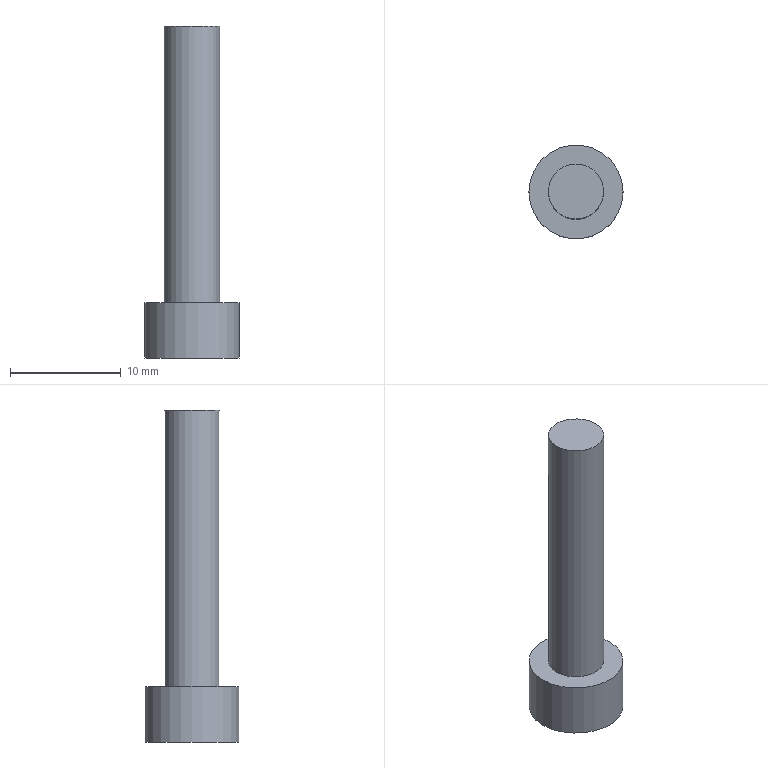Part | STEP file | 1 solid | 12 faces | box 8.5 x 8.5 x 30 mm | volume 728.873 mm3 | plane 10 | cylinder 2 | commonest cylinder face diameters 5 x1 8.5 x1
STEP:
#1=CARTESIAN_POINT('',(0.,0.,0.));
#2=DIRECTION('',(0.,0.,1.));
#3=DIRECTION('',(1.,0.,0.));
#4=AXIS2_PLACEMENT_3D('',#1,#2,#3);
#5=CARTESIAN_POINT('',(1182.997,385.855,-56.381));
#6=VERTEX_POINT('',#5);
#7=CARTESIAN_POINT('',(1187.247,385.855,-56.381));
#8=DIRECTION('',(0.,0.,-1.));
#9=DIRECTION('',(-1.,0.,0.));
#10=AXIS2_PLACEMENT_3D('',#7,#8,#9);
#11=CIRCLE('',#10,4.25);
#12=CARTESIAN_POINT('',(1182.997,385.855,-56.381));
#13=DIRECTION('',(0.,0.,1.));
#14=DIRECTION('',(1.,0.,0.));
#15=AXIS2_PLACEMENT_3D('',#12,#13,#14);
#16=PLANE('',#15);
#17=CARTESIAN_POINT('',(0.,0.));
#18=CARTESIAN_POINT('',(0.,7.361));
#19=CARTESIAN_POINT('',(6.375,3.681));
#20=CARTESIAN_POINT('',(12.75,0.));
#21=CARTESIAN_POINT('',(6.375,-3.681));
#22=CARTESIAN_POINT('',(0.,-7.361));
#23=CARTESIAN_POINT('',(0.,0.));
#24=(BOUNDED_CURVE()B_SPLINE_CURVE(2,(#17,#18,#19,#20,#21,#22,#23),.UNSPECIFIED.,.T.,.F.)B_SPLINE_CURVE_WITH_KNOTS((1,2,2,2,2,1),(-2.094,0.,2.094,4.189,6.283,8.378),.UNSPECIFIED.)CURVE()GEOMETRIC_REPRESENTATION_ITEM()RATIONAL_B_SPLINE_CURVE((1.,0.5,1.,0.5,1.,0.5,1.))REPRESENTATION_ITEM(''));
#25=(GEOMETRIC_REPRESENTATION_CONTEXT(2)PARAMETRIC_REPRESENTATION_CONTEXT()REPRESENTATION_CONTEXT('',''));
#26=DEFINITIONAL_REPRESENTATION('',(#24),#25);
#27=PCURVE('',#16,#26);
#28=CARTESIAN_POINT('',(1187.247,385.855,-19.981));
#29=DIRECTION('',(0.,0.,-1.));
#30=DIRECTION('',(-1.,0.,0.));
#31=AXIS2_PLACEMENT_3D('',#28,#29,#30);
#32=CYLINDRICAL_SURFACE('',#31,4.25);
#33=CARTESIAN_POINT('',(0.,36.4));
#34=DIRECTION('',(1.,0.));
#35=VECTOR('',#34,1.);
#36=LINE('',#33,#35);
#37=(GEOMETRIC_REPRESENTATION_CONTEXT(2)PARAMETRIC_REPRESENTATION_CONTEXT()REPRESENTATION_CONTEXT('',''));
#38=DEFINITIONAL_REPRESENTATION('',(#36),#37);
#39=PCURVE('',#32,#38);
#40=SURFACE_CURVE('',#11,(#27,#39),.PCURVE_S1.);
#41=EDGE_CURVE('',#6,#6,#40,.T.);
#42=ORIENTED_EDGE('',*,*,#41,.T.);
#43=EDGE_LOOP('',(#42));
#44=FACE_BOUND('',#43,.T.);
#45=CARTESIAN_POINT('',(1188.402,387.855,-56.381));
#46=VERTEX_POINT('',#45);
#47=CARTESIAN_POINT('',(1186.092,387.855,-56.381));
#48=VERTEX_POINT('',#47);
#49=CARTESIAN_POINT('',(1188.402,387.855,-56.381));
#50=DIRECTION('',(-1.,0.,0.));
#51=VECTOR('',#50,1.);
#52=LINE('',#49,#51);
#53=CARTESIAN_POINT('',(5.405,2.));
#54=DIRECTION('',(-1.,0.));
#55=VECTOR('',#54,1.);
#56=LINE('',#53,#55);
#57=(GEOMETRIC_REPRESENTATION_CONTEXT(2)PARAMETRIC_REPRESENTATION_CONTEXT()REPRESENTATION_CONTEXT('',''));
#58=DEFINITIONAL_REPRESENTATION('',(#56),#57);
#59=PCURVE('',#16,#58);
#60=CARTESIAN_POINT('',(1188.402,387.855,-53.081));
#61=DIRECTION('',(0.,-1.,0.));
#62=DIRECTION('',(-1.,0.,0.));
#63=AXIS2_PLACEMENT_3D('',#60,#61,#62);
#64=PLANE('',#63);
#65=CARTESIAN_POINT('',(0.,3.3));
#66=DIRECTION('',(1.,0.));
#67=VECTOR('',#66,1.);
#68=LINE('',#65,#67);
#69=(GEOMETRIC_REPRESENTATION_CONTEXT(2)PARAMETRIC_REPRESENTATION_CONTEXT()REPRESENTATION_CONTEXT('',''));
#70=DEFINITIONAL_REPRESENTATION('',(#68),#69);
#71=PCURVE('',#64,#70);
#72=SURFACE_CURVE('',#52,(#59,#71),.PCURVE_S1.);
#73=EDGE_CURVE('',#46,#48,#72,.T.);
#74=ORIENTED_EDGE('',*,*,#73,.T.);
#75=CARTESIAN_POINT('',(1184.938,385.855,-56.381));
#76=VERTEX_POINT('',#75);
#77=CARTESIAN_POINT('',(1186.092,387.855,-56.381));
#78=DIRECTION('',(-0.5,-0.866,0.));
#79=VECTOR('',#78,1.);
#80=LINE('',#77,#79);
#81=CARTESIAN_POINT('',(3.095,2.));
#82=DIRECTION('',(-0.5,-0.866));
#83=VECTOR('',#82,1.);
#84=LINE('',#81,#83);
#85=(GEOMETRIC_REPRESENTATION_CONTEXT(2)PARAMETRIC_REPRESENTATION_CONTEXT()REPRESENTATION_CONTEXT('',''));
#86=DEFINITIONAL_REPRESENTATION('',(#84),#85);
#87=PCURVE('',#16,#86);
#88=CARTESIAN_POINT('',(1186.092,387.855,-53.081));
#89=DIRECTION('',(0.866,-0.5,0.));
#90=DIRECTION('',(-0.5,-0.866,0.));
#91=AXIS2_PLACEMENT_3D('',#88,#89,#90);
#92=PLANE('',#91);
#93=CARTESIAN_POINT('',(0.,3.3));
#94=DIRECTION('',(1.,0.));
#95=VECTOR('',#94,1.);
#96=LINE('',#93,#95);
#97=(GEOMETRIC_REPRESENTATION_CONTEXT(2)PARAMETRIC_REPRESENTATION_CONTEXT()REPRESENTATION_CONTEXT('',''));
#98=DEFINITIONAL_REPRESENTATION('',(#96),#97);
#99=PCURVE('',#92,#98);
#100=SURFACE_CURVE('',#80,(#87,#99),.PCURVE_S1.);
#101=EDGE_CURVE('',#48,#76,#100,.T.);
#102=ORIENTED_EDGE('',*,*,#101,.T.);
#103=CARTESIAN_POINT('',(1186.092,383.855,-56.381));
#104=VERTEX_POINT('',#103);
#105=CARTESIAN_POINT('',(1184.938,385.855,-56.381));
#106=DIRECTION('',(0.5,-0.866,0.));
#107=VECTOR('',#106,1.);
#108=LINE('',#105,#107);
#109=CARTESIAN_POINT('',(1.941,0.));
#110=DIRECTION('',(0.5,-0.866));
#111=VECTOR('',#110,1.);
#112=LINE('',#109,#111);
#113=(GEOMETRIC_REPRESENTATION_CONTEXT(2)PARAMETRIC_REPRESENTATION_CONTEXT()REPRESENTATION_CONTEXT('',''));
#114=DEFINITIONAL_REPRESENTATION('',(#112),#113);
#115=PCURVE('',#16,#114);
#116=CARTESIAN_POINT('',(1184.938,385.855,-53.081));
#117=DIRECTION('',(0.866,0.5,0.));
#118=DIRECTION('',(0.5,-0.866,0.));
#119=AXIS2_PLACEMENT_3D('',#116,#117,#118);
#120=PLANE('',#119);
#121=CARTESIAN_POINT('',(0.,3.3));
#122=DIRECTION('',(1.,0.));
#123=VECTOR('',#122,1.);
#124=LINE('',#121,#123);
#125=(GEOMETRIC_REPRESENTATION_CONTEXT(2)PARAMETRIC_REPRESENTATION_CONTEXT()REPRESENTATION_CONTEXT('',''));
#126=DEFINITIONAL_REPRESENTATION('',(#124),#125);
#127=PCURVE('',#120,#126);
#128=SURFACE_CURVE('',#108,(#115,#127),.PCURVE_S1.);
#129=EDGE_CURVE('',#76,#104,#128,.T.);
#130=ORIENTED_EDGE('',*,*,#129,.T.);
#131=CARTESIAN_POINT('',(1188.402,383.855,-56.381));
#132=VERTEX_POINT('',#131);
#133=CARTESIAN_POINT('',(1186.092,383.855,-56.381));
#134=DIRECTION('',(1.,0.,0.));
#135=VECTOR('',#134,1.);
#136=LINE('',#133,#135);
#137=CARTESIAN_POINT('',(3.095,-2.));
#138=DIRECTION('',(1.,0.));
#139=VECTOR('',#138,1.);
#140=LINE('',#137,#139);
#141=(GEOMETRIC_REPRESENTATION_CONTEXT(2)PARAMETRIC_REPRESENTATION_CONTEXT()REPRESENTATION_CONTEXT('',''));
#142=DEFINITIONAL_REPRESENTATION('',(#140),#141);
#143=PCURVE('',#16,#142);
#144=CARTESIAN_POINT('',(1186.092,383.855,-53.081));
#145=DIRECTION('',(0.,1.,0.));
#146=DIRECTION('',(0.,0.,-1.));
#147=AXIS2_PLACEMENT_3D('',#144,#145,#146);
#148=PLANE('',#147);
#149=CARTESIAN_POINT('',(3.3,0.));
#150=DIRECTION('',(0.,-1.));
#151=VECTOR('',#150,1.);
#152=LINE('',#149,#151);
#153=(GEOMETRIC_REPRESENTATION_CONTEXT(2)PARAMETRIC_REPRESENTATION_CONTEXT()REPRESENTATION_CONTEXT('',''));
#154=DEFINITIONAL_REPRESENTATION('',(#152),#153);
#155=PCURVE('',#148,#154);
#156=SURFACE_CURVE('',#136,(#143,#155),.PCURVE_S1.);
#157=EDGE_CURVE('',#104,#132,#156,.T.);
#158=ORIENTED_EDGE('',*,*,#157,.T.);
#159=CARTESIAN_POINT('',(1189.557,385.855,-56.381));
#160=VERTEX_POINT('',#159);
#161=CARTESIAN_POINT('',(1188.402,383.855,-56.381));
#162=DIRECTION('',(0.5,0.866,0.));
#163=VECTOR('',#162,1.);
#164=LINE('',#161,#163);
#165=CARTESIAN_POINT('',(5.405,-2.));
#166=DIRECTION('',(0.5,0.866));
#167=VECTOR('',#166,1.);
#168=LINE('',#165,#167);
#169=(GEOMETRIC_REPRESENTATION_CONTEXT(2)PARAMETRIC_REPRESENTATION_CONTEXT()REPRESENTATION_CONTEXT('',''));
#170=DEFINITIONAL_REPRESENTATION('',(#168),#169);
#171=PCURVE('',#16,#170);
#172=CARTESIAN_POINT('',(1188.402,383.855,-53.081));
#173=DIRECTION('',(-0.866,0.5,0.));
#174=DIRECTION('',(0.5,0.866,0.));
#175=AXIS2_PLACEMENT_3D('',#172,#173,#174);
#176=PLANE('',#175);
#177=CARTESIAN_POINT('',(0.,3.3));
#178=DIRECTION('',(1.,0.));
#179=VECTOR('',#178,1.);
#180=LINE('',#177,#179);
#181=(GEOMETRIC_REPRESENTATION_CONTEXT(2)PARAMETRIC_REPRESENTATION_CONTEXT()REPRESENTATION_CONTEXT('',''));
#182=DEFINITIONAL_REPRESENTATION('',(#180),#181);
#183=PCURVE('',#176,#182);
#184=SURFACE_CURVE('',#164,(#171,#183),.PCURVE_S1.);
#185=EDGE_CURVE('',#132,#160,#184,.T.);
#186=ORIENTED_EDGE('',*,*,#185,.T.);
#187=CARTESIAN_POINT('',(1189.557,385.855,-56.381));
#188=DIRECTION('',(-0.5,0.866,0.));
#189=VECTOR('',#188,1.);
#190=LINE('',#187,#189);
#191=CARTESIAN_POINT('',(6.559,0.));
#192=DIRECTION('',(-0.5,0.866));
#193=VECTOR('',#192,1.);
#194=LINE('',#191,#193);
#195=(GEOMETRIC_REPRESENTATION_CONTEXT(2)PARAMETRIC_REPRESENTATION_CONTEXT()REPRESENTATION_CONTEXT('',''));
#196=DEFINITIONAL_REPRESENTATION('',(#194),#195);
#197=PCURVE('',#16,#196);
#198=CARTESIAN_POINT('',(1189.557,385.855,-53.081));
#199=DIRECTION('',(-0.866,-0.5,0.));
#200=DIRECTION('',(-0.5,0.866,0.));
#201=AXIS2_PLACEMENT_3D('',#198,#199,#200);
#202=PLANE('',#201);
#203=CARTESIAN_POINT('',(0.,3.3));
#204=DIRECTION('',(1.,0.));
#205=VECTOR('',#204,1.);
#206=LINE('',#203,#205);
#207=(GEOMETRIC_REPRESENTATION_CONTEXT(2)PARAMETRIC_REPRESENTATION_CONTEXT()REPRESENTATION_CONTEXT('',''));
#208=DEFINITIONAL_REPRESENTATION('',(#206),#207);
#209=PCURVE('',#202,#208);
#210=SURFACE_CURVE('',#190,(#197,#209),.PCURVE_S1.);
#211=EDGE_CURVE('',#160,#46,#210,.T.);
#212=ORIENTED_EDGE('',*,*,#211,.T.);
#213=EDGE_LOOP('',(#74,#102,#130,#158,#186,#212));
#214=FACE_BOUND('',#213,.T.);
#215=ADVANCED_FACE('',(#44,#214),#16,.F.);
#216=ORIENTED_EDGE('',*,*,#41,.F.);
#217=CARTESIAN_POINT('',(1182.997,385.855,-51.381));
#218=VERTEX_POINT('',#217);
#219=CARTESIAN_POINT('',(1182.997,385.855,-51.381));
#220=CARTESIAN_POINT('',(1182.997,385.855,-56.381));
#221=B_SPLINE_CURVE_WITH_KNOTS('',1,(#219,#220),.UNSPECIFIED.,.F.,.F.,(2,2),(31.4,36.4),.PIECEWISE_BEZIER_KNOTS.);
#222=CARTESIAN_POINT('',(0.,0.));
#223=DIRECTION('',(0.,1.));
#224=VECTOR('',#223,1.);
#225=LINE('',#222,#224);
#226=(GEOMETRIC_REPRESENTATION_CONTEXT(2)PARAMETRIC_REPRESENTATION_CONTEXT()REPRESENTATION_CONTEXT('',''));
#227=DEFINITIONAL_REPRESENTATION('',(#225),#226);
#228=PCURVE('',#32,#227);
#229=CARTESIAN_POINT('',(6.283,0.));
#230=DIRECTION('',(0.,1.));
#231=VECTOR('',#230,1.);
#232=LINE('',#229,#231);
#233=(GEOMETRIC_REPRESENTATION_CONTEXT(2)PARAMETRIC_REPRESENTATION_CONTEXT()REPRESENTATION_CONTEXT('',''));
#234=DEFINITIONAL_REPRESENTATION('',(#232),#233);
#235=PCURVE('',#32,#234);
#236=SEAM_CURVE('',#221,(#228,#235),.PCURVE_S1.);
#237=EDGE_CURVE('',#218,#6,#236,.T.);
#238=ORIENTED_EDGE('',*,*,#237,.F.);
#239=CARTESIAN_POINT('',(1187.247,385.855,-51.381));
#240=DIRECTION('',(0.,0.,-1.));
#241=DIRECTION('',(-1.,0.,0.));
#242=AXIS2_PLACEMENT_3D('',#239,#240,#241);
#243=CIRCLE('',#242,4.25);
#244=CARTESIAN_POINT('',(0.,31.4));
#245=DIRECTION('',(1.,0.));
#246=VECTOR('',#245,1.);
#247=LINE('',#244,#246);
#248=(GEOMETRIC_REPRESENTATION_CONTEXT(2)PARAMETRIC_REPRESENTATION_CONTEXT()REPRESENTATION_CONTEXT('',''));
#249=DEFINITIONAL_REPRESENTATION('',(#247),#248);
#250=PCURVE('',#32,#249);
#251=CARTESIAN_POINT('',(1184.747,385.855,-51.381));
#252=DIRECTION('',(0.,0.,-1.));
#253=DIRECTION('',(-1.,0.,0.));
#254=AXIS2_PLACEMENT_3D('',#251,#252,#253);
#255=PLANE('',#254);
#256=CARTESIAN_POINT('',(-2.5,0.));
#257=DIRECTION('',(1.,0.));
#258=AXIS2_PLACEMENT_2D('',#256,#257);
#259=CIRCLE('',#258,4.25);
#260=(GEOMETRIC_REPRESENTATION_CONTEXT(2)PARAMETRIC_REPRESENTATION_CONTEXT()REPRESENTATION_CONTEXT('',''));
#261=DEFINITIONAL_REPRESENTATION('',(#259),#260);
#262=PCURVE('',#255,#261);
#263=SURFACE_CURVE('',#243,(#250,#262),.PCURVE_S1.);
#264=EDGE_CURVE('',#218,#218,#263,.T.);
#265=ORIENTED_EDGE('',*,*,#264,.T.);
#266=ORIENTED_EDGE('',*,*,#237,.T.);
#267=EDGE_LOOP('',(#216,#238,#265,#266));
#268=FACE_BOUND('',#267,.T.);
#269=ADVANCED_FACE('',(#268),#32,.T.);
#270=ORIENTED_EDGE('',*,*,#264,.F.);
#271=EDGE_LOOP('',(#270));
#272=FACE_BOUND('',#271,.T.);
#273=CARTESIAN_POINT('',(1184.747,385.855,-51.381));
#274=VERTEX_POINT('',#273);
#275=CARTESIAN_POINT('',(1187.247,385.855,-51.381));
#276=DIRECTION('',(0.,0.,-1.));
#277=DIRECTION('',(-1.,0.,0.));
#278=AXIS2_PLACEMENT_3D('',#275,#276,#277);
#279=CIRCLE('',#278,2.5);
#280=CARTESIAN_POINT('',(-2.5,0.));
#281=DIRECTION('',(1.,0.));
#282=AXIS2_PLACEMENT_2D('',#280,#281);
#283=CIRCLE('',#282,2.5);
#284=(GEOMETRIC_REPRESENTATION_CONTEXT(2)PARAMETRIC_REPRESENTATION_CONTEXT()REPRESENTATION_CONTEXT('',''));
#285=DEFINITIONAL_REPRESENTATION('',(#283),#284);
#286=PCURVE('',#255,#285);
#287=CARTESIAN_POINT('',(1187.247,385.855,-19.981));
#288=DIRECTION('',(0.,0.,-1.));
#289=DIRECTION('',(-1.,0.,0.));
#290=AXIS2_PLACEMENT_3D('',#287,#288,#289);
#291=CYLINDRICAL_SURFACE('',#290,2.5);
#292=CARTESIAN_POINT('',(0.,31.4));
#293=DIRECTION('',(1.,0.));
#294=VECTOR('',#293,1.);
#295=LINE('',#292,#294);
#296=(GEOMETRIC_REPRESENTATION_CONTEXT(2)PARAMETRIC_REPRESENTATION_CONTEXT()REPRESENTATION_CONTEXT('',''));
#297=DEFINITIONAL_REPRESENTATION('',(#295),#296);
#298=PCURVE('',#291,#297);
#299=SURFACE_CURVE('',#279,(#286,#298),.PCURVE_S1.);
#300=EDGE_CURVE('',#274,#274,#299,.T.);
#301=ORIENTED_EDGE('',*,*,#300,.T.);
#302=EDGE_LOOP('',(#301));
#303=FACE_BOUND('',#302,.T.);
#304=ADVANCED_FACE('',(#272,#303),#255,.F.);
#305=ORIENTED_EDGE('',*,*,#300,.F.);
#306=CARTESIAN_POINT('',(1184.747,385.855,-26.381));
#307=VERTEX_POINT('',#306);
#308=CARTESIAN_POINT('',(1184.747,385.855,-26.381));
#309=CARTESIAN_POINT('',(1184.747,385.855,-51.381));
#310=B_SPLINE_CURVE_WITH_KNOTS('',1,(#308,#309),.UNSPECIFIED.,.F.,.F.,(2,2),(6.4,31.4),.PIECEWISE_BEZIER_KNOTS.);
#311=CARTESIAN_POINT('',(0.,0.));
#312=DIRECTION('',(0.,1.));
#313=VECTOR('',#312,1.);
#314=LINE('',#311,#313);
#315=(GEOMETRIC_REPRESENTATION_CONTEXT(2)PARAMETRIC_REPRESENTATION_CONTEXT()REPRESENTATION_CONTEXT('',''));
#316=DEFINITIONAL_REPRESENTATION('',(#314),#315);
#317=PCURVE('',#291,#316);
#318=CARTESIAN_POINT('',(6.283,0.));
#319=DIRECTION('',(0.,1.));
#320=VECTOR('',#319,1.);
#321=LINE('',#318,#320);
#322=(GEOMETRIC_REPRESENTATION_CONTEXT(2)PARAMETRIC_REPRESENTATION_CONTEXT()REPRESENTATION_CONTEXT('',''));
#323=DEFINITIONAL_REPRESENTATION('',(#321),#322);
#324=PCURVE('',#291,#323);
#325=SEAM_CURVE('',#310,(#317,#324),.PCURVE_S1.);
#326=EDGE_CURVE('',#307,#274,#325,.T.);
#327=ORIENTED_EDGE('',*,*,#326,.F.);
#328=CARTESIAN_POINT('',(1187.247,385.855,-26.381));
#329=DIRECTION('',(0.,0.,-1.));
#330=DIRECTION('',(-1.,0.,0.));
#331=AXIS2_PLACEMENT_3D('',#328,#329,#330);
#332=CIRCLE('',#331,2.5);
#333=CARTESIAN_POINT('',(0.,6.4));
#334=DIRECTION('',(1.,0.));
#335=VECTOR('',#334,1.);
#336=LINE('',#333,#335);
#337=(GEOMETRIC_REPRESENTATION_CONTEXT(2)PARAMETRIC_REPRESENTATION_CONTEXT()REPRESENTATION_CONTEXT('',''));
#338=DEFINITIONAL_REPRESENTATION('',(#336),#337);
#339=PCURVE('',#291,#338);
#340=CARTESIAN_POINT('',(1187.247,385.855,-26.381));
#341=DIRECTION('',(0.,0.,-1.));
#342=DIRECTION('',(-1.,0.,0.));
#343=AXIS2_PLACEMENT_3D('',#340,#341,#342);
#344=PLANE('',#343);
#345=CARTESIAN_POINT('',(0.,0.));
#346=DIRECTION('',(1.,0.));
#347=AXIS2_PLACEMENT_2D('',#345,#346);
#348=CIRCLE('',#347,2.5);
#349=(GEOMETRIC_REPRESENTATION_CONTEXT(2)PARAMETRIC_REPRESENTATION_CONTEXT()REPRESENTATION_CONTEXT('',''));
#350=DEFINITIONAL_REPRESENTATION('',(#348),#349);
#351=PCURVE('',#344,#350);
#352=SURFACE_CURVE('',#332,(#339,#351),.PCURVE_S1.);
#353=EDGE_CURVE('',#307,#307,#352,.T.);
#354=ORIENTED_EDGE('',*,*,#353,.T.);
#355=ORIENTED_EDGE('',*,*,#326,.T.);
#356=EDGE_LOOP('',(#305,#327,#354,#355));
#357=FACE_BOUND('',#356,.T.);
#358=ADVANCED_FACE('',(#357),#291,.T.);
#359=ORIENTED_EDGE('',*,*,#353,.F.);
#360=EDGE_LOOP('',(#359));
#361=FACE_BOUND('',#360,.T.);
#362=ADVANCED_FACE('',(#361),#344,.F.);
#363=ORIENTED_EDGE('',*,*,#73,.F.);
#364=CARTESIAN_POINT('',(1188.402,387.855,-53.081));
#365=VERTEX_POINT('',#364);
#366=CARTESIAN_POINT('',(1188.402,387.855,-53.081));
#367=DIRECTION('',(0.,0.,1.));
#368=VECTOR('',#367,1.);
#369=LINE('',#366,#368);
#370=CARTESIAN_POINT('',(0.,0.));
#371=DIRECTION('',(0.,-1.));
#372=VECTOR('',#371,1.);
#373=LINE('',#370,#372);
#374=(GEOMETRIC_REPRESENTATION_CONTEXT(2)PARAMETRIC_REPRESENTATION_CONTEXT()REPRESENTATION_CONTEXT('',''));
#375=DEFINITIONAL_REPRESENTATION('',(#373),#374);
#376=PCURVE('',#64,#375);
#377=CARTESIAN_POINT('',(2.309,0.));
#378=DIRECTION('',(0.,-1.));
#379=VECTOR('',#378,1.);
#380=LINE('',#377,#379);
#381=(GEOMETRIC_REPRESENTATION_CONTEXT(2)PARAMETRIC_REPRESENTATION_CONTEXT()REPRESENTATION_CONTEXT('',''));
#382=DEFINITIONAL_REPRESENTATION('',(#380),#381);
#383=PCURVE('',#202,#382);
#384=SURFACE_CURVE('',#369,(#376,#383),.PCURVE_S1.);
#385=EDGE_CURVE('',#46,#365,#384,.T.);
#386=ORIENTED_EDGE('',*,*,#385,.T.);
#387=CARTESIAN_POINT('',(1186.092,387.855,-53.081));
#388=VERTEX_POINT('',#387);
#389=CARTESIAN_POINT('',(1188.402,387.855,-53.081));
#390=DIRECTION('',(1.,0.,0.));
#391=VECTOR('',#390,1.);
#392=LINE('',#389,#391);
#393=CARTESIAN_POINT('',(0.,0.));
#394=DIRECTION('',(-1.,0.));
#395=VECTOR('',#394,1.);
#396=LINE('',#393,#395);
#397=(GEOMETRIC_REPRESENTATION_CONTEXT(2)PARAMETRIC_REPRESENTATION_CONTEXT()REPRESENTATION_CONTEXT('',''));
#398=DEFINITIONAL_REPRESENTATION('',(#396),#397);
#399=PCURVE('',#64,#398);
#400=CARTESIAN_POINT('',(1187.247,385.855,-53.081));
#401=DIRECTION('',(0.,0.,1.));
#402=DIRECTION('',(1.,0.,0.));
#403=AXIS2_PLACEMENT_3D('',#400,#401,#402);
#404=PLANE('',#403);
#405=CARTESIAN_POINT('',(1.155,2.));
#406=DIRECTION('',(1.,0.));
#407=VECTOR('',#406,1.);
#408=LINE('',#405,#407);
#409=(GEOMETRIC_REPRESENTATION_CONTEXT(2)PARAMETRIC_REPRESENTATION_CONTEXT()REPRESENTATION_CONTEXT('',''));
#410=DEFINITIONAL_REPRESENTATION('',(#408),#409);
#411=PCURVE('',#404,#410);
#412=SURFACE_CURVE('',#392,(#399,#411),.PCURVE_S1.);
#413=EDGE_CURVE('',#388,#365,#412,.T.);
#414=ORIENTED_EDGE('',*,*,#413,.F.);
#415=CARTESIAN_POINT('',(1186.092,387.855,-53.081));
#416=DIRECTION('',(0.,0.,1.));
#417=VECTOR('',#416,1.);
#418=LINE('',#415,#417);
#419=CARTESIAN_POINT('',(2.309,0.));
#420=DIRECTION('',(0.,-1.));
#421=VECTOR('',#420,1.);
#422=LINE('',#419,#421);
#423=(GEOMETRIC_REPRESENTATION_CONTEXT(2)PARAMETRIC_REPRESENTATION_CONTEXT()REPRESENTATION_CONTEXT('',''));
#424=DEFINITIONAL_REPRESENTATION('',(#422),#423);
#425=PCURVE('',#64,#424);
#426=CARTESIAN_POINT('',(0.,0.));
#427=DIRECTION('',(0.,-1.));
#428=VECTOR('',#427,1.);
#429=LINE('',#426,#428);
#430=(GEOMETRIC_REPRESENTATION_CONTEXT(2)PARAMETRIC_REPRESENTATION_CONTEXT()REPRESENTATION_CONTEXT('',''));
#431=DEFINITIONAL_REPRESENTATION('',(#429),#430);
#432=PCURVE('',#92,#431);
#433=SURFACE_CURVE('',#418,(#425,#432),.PCURVE_S1.);
#434=EDGE_CURVE('',#48,#388,#433,.T.);
#435=ORIENTED_EDGE('',*,*,#434,.F.);
#436=EDGE_LOOP('',(#363,#386,#414,#435));
#437=FACE_BOUND('',#436,.T.);
#438=ADVANCED_FACE('',(#437),#64,.T.);
#439=ORIENTED_EDGE('',*,*,#101,.F.);
#440=ORIENTED_EDGE('',*,*,#434,.T.);
#441=CARTESIAN_POINT('',(1184.938,385.855,-53.081));
#442=VERTEX_POINT('',#441);
#443=CARTESIAN_POINT('',(1186.092,387.855,-53.081));
#444=DIRECTION('',(0.5,0.866,0.));
#445=VECTOR('',#444,1.);
#446=LINE('',#443,#445);
#447=CARTESIAN_POINT('',(0.,0.));
#448=DIRECTION('',(-1.,0.));
#449=VECTOR('',#448,1.);
#450=LINE('',#447,#449);
#451=(GEOMETRIC_REPRESENTATION_CONTEXT(2)PARAMETRIC_REPRESENTATION_CONTEXT()REPRESENTATION_CONTEXT('',''));
#452=DEFINITIONAL_REPRESENTATION('',(#450),#451);
#453=PCURVE('',#92,#452);
#454=CARTESIAN_POINT('',(-1.155,2.));
#455=DIRECTION('',(0.5,0.866));
#456=VECTOR('',#455,1.);
#457=LINE('',#454,#456);
#458=(GEOMETRIC_REPRESENTATION_CONTEXT(2)PARAMETRIC_REPRESENTATION_CONTEXT()REPRESENTATION_CONTEXT('',''));
#459=DEFINITIONAL_REPRESENTATION('',(#457),#458);
#460=PCURVE('',#404,#459);
#461=SURFACE_CURVE('',#446,(#453,#460),.PCURVE_S1.);
#462=EDGE_CURVE('',#442,#388,#461,.T.);
#463=ORIENTED_EDGE('',*,*,#462,.F.);
#464=CARTESIAN_POINT('',(1184.938,385.855,-53.081));
#465=DIRECTION('',(0.,0.,1.));
#466=VECTOR('',#465,1.);
#467=LINE('',#464,#466);
#468=CARTESIAN_POINT('',(2.309,0.));
#469=DIRECTION('',(0.,-1.));
#470=VECTOR('',#469,1.);
#471=LINE('',#468,#470);
#472=(GEOMETRIC_REPRESENTATION_CONTEXT(2)PARAMETRIC_REPRESENTATION_CONTEXT()REPRESENTATION_CONTEXT('',''));
#473=DEFINITIONAL_REPRESENTATION('',(#471),#472);
#474=PCURVE('',#92,#473);
#475=CARTESIAN_POINT('',(0.,0.));
#476=DIRECTION('',(0.,-1.));
#477=VECTOR('',#476,1.);
#478=LINE('',#475,#477);
#479=(GEOMETRIC_REPRESENTATION_CONTEXT(2)PARAMETRIC_REPRESENTATION_CONTEXT()REPRESENTATION_CONTEXT('',''));
#480=DEFINITIONAL_REPRESENTATION('',(#478),#479);
#481=PCURVE('',#120,#480);
#482=SURFACE_CURVE('',#467,(#474,#481),.PCURVE_S1.);
#483=EDGE_CURVE('',#76,#442,#482,.T.);
#484=ORIENTED_EDGE('',*,*,#483,.F.);
#485=EDGE_LOOP('',(#439,#440,#463,#484));
#486=FACE_BOUND('',#485,.T.);
#487=ADVANCED_FACE('',(#486),#92,.T.);
#488=ORIENTED_EDGE('',*,*,#129,.F.);
#489=ORIENTED_EDGE('',*,*,#483,.T.);
#490=CARTESIAN_POINT('',(1186.092,383.855,-53.081));
#491=VERTEX_POINT('',#490);
#492=CARTESIAN_POINT('',(1184.938,385.855,-53.081));
#493=DIRECTION('',(-0.5,0.866,0.));
#494=VECTOR('',#493,1.);
#495=LINE('',#492,#494);
#496=CARTESIAN_POINT('',(0.,0.));
#497=DIRECTION('',(-1.,0.));
#498=VECTOR('',#497,1.);
#499=LINE('',#496,#498);
#500=(GEOMETRIC_REPRESENTATION_CONTEXT(2)PARAMETRIC_REPRESENTATION_CONTEXT()REPRESENTATION_CONTEXT('',''));
#501=DEFINITIONAL_REPRESENTATION('',(#499),#500);
#502=PCURVE('',#120,#501);
#503=CARTESIAN_POINT('',(-2.309,0.));
#504=DIRECTION('',(-0.5,0.866));
#505=VECTOR('',#504,1.);
#506=LINE('',#503,#505);
#507=(GEOMETRIC_REPRESENTATION_CONTEXT(2)PARAMETRIC_REPRESENTATION_CONTEXT()REPRESENTATION_CONTEXT('',''));
#508=DEFINITIONAL_REPRESENTATION('',(#506),#507);
#509=PCURVE('',#404,#508);
#510=SURFACE_CURVE('',#495,(#502,#509),.PCURVE_S1.);
#511=EDGE_CURVE('',#491,#442,#510,.T.);
#512=ORIENTED_EDGE('',*,*,#511,.F.);
#513=CARTESIAN_POINT('',(1186.092,383.855,-53.081));
#514=DIRECTION('',(0.,0.,1.));
#515=VECTOR('',#514,1.);
#516=LINE('',#513,#515);
#517=CARTESIAN_POINT('',(2.309,0.));
#518=DIRECTION('',(0.,-1.));
#519=VECTOR('',#518,1.);
#520=LINE('',#517,#519);
#521=(GEOMETRIC_REPRESENTATION_CONTEXT(2)PARAMETRIC_REPRESENTATION_CONTEXT()REPRESENTATION_CONTEXT('',''));
#522=DEFINITIONAL_REPRESENTATION('',(#520),#521);
#523=PCURVE('',#120,#522);
#524=CARTESIAN_POINT('',(0.,0.));
#525=DIRECTION('',(-1.,0.));
#526=VECTOR('',#525,1.);
#527=LINE('',#524,#526);
#528=(GEOMETRIC_REPRESENTATION_CONTEXT(2)PARAMETRIC_REPRESENTATION_CONTEXT()REPRESENTATION_CONTEXT('',''));
#529=DEFINITIONAL_REPRESENTATION('',(#527),#528);
#530=PCURVE('',#148,#529);
#531=SURFACE_CURVE('',#516,(#523,#530),.PCURVE_S1.);
#532=EDGE_CURVE('',#104,#491,#531,.T.);
#533=ORIENTED_EDGE('',*,*,#532,.F.);
#534=EDGE_LOOP('',(#488,#489,#512,#533));
#535=FACE_BOUND('',#534,.T.);
#536=ADVANCED_FACE('',(#535),#120,.T.);
#537=ORIENTED_EDGE('',*,*,#157,.F.);
#538=ORIENTED_EDGE('',*,*,#532,.T.);
#539=CARTESIAN_POINT('',(1188.402,383.855,-53.081));
#540=VERTEX_POINT('',#539);
#541=CARTESIAN_POINT('',(1186.092,383.855,-53.081));
#542=DIRECTION('',(-1.,0.,0.));
#543=VECTOR('',#542,1.);
#544=LINE('',#541,#543);
#545=CARTESIAN_POINT('',(0.,0.));
#546=DIRECTION('',(0.,1.));
#547=VECTOR('',#546,1.);
#548=LINE('',#545,#547);
#549=(GEOMETRIC_REPRESENTATION_CONTEXT(2)PARAMETRIC_REPRESENTATION_CONTEXT()REPRESENTATION_CONTEXT('',''));
#550=DEFINITIONAL_REPRESENTATION('',(#548),#549);
#551=PCURVE('',#148,#550);
#552=CARTESIAN_POINT('',(-1.155,-2.));
#553=DIRECTION('',(-1.,0.));
#554=VECTOR('',#553,1.);
#555=LINE('',#552,#554);
#556=(GEOMETRIC_REPRESENTATION_CONTEXT(2)PARAMETRIC_REPRESENTATION_CONTEXT()REPRESENTATION_CONTEXT('',''));
#557=DEFINITIONAL_REPRESENTATION('',(#555),#556);
#558=PCURVE('',#404,#557);
#559=SURFACE_CURVE('',#544,(#551,#558),.PCURVE_S1.);
#560=EDGE_CURVE('',#540,#491,#559,.T.);
#561=ORIENTED_EDGE('',*,*,#560,.F.);
#562=CARTESIAN_POINT('',(1188.402,383.855,-53.081));
#563=DIRECTION('',(0.,0.,1.));
#564=VECTOR('',#563,1.);
#565=LINE('',#562,#564);
#566=CARTESIAN_POINT('',(0.,-2.309));
#567=DIRECTION('',(-1.,0.));
#568=VECTOR('',#567,1.);
#569=LINE('',#566,#568);
#570=(GEOMETRIC_REPRESENTATION_CONTEXT(2)PARAMETRIC_REPRESENTATION_CONTEXT()REPRESENTATION_CONTEXT('',''));
#571=DEFINITIONAL_REPRESENTATION('',(#569),#570);
#572=PCURVE('',#148,#571);
#573=CARTESIAN_POINT('',(0.,0.));
#574=DIRECTION('',(0.,-1.));
#575=VECTOR('',#574,1.);
#576=LINE('',#573,#575);
#577=(GEOMETRIC_REPRESENTATION_CONTEXT(2)PARAMETRIC_REPRESENTATION_CONTEXT()REPRESENTATION_CONTEXT('',''));
#578=DEFINITIONAL_REPRESENTATION('',(#576),#577);
#579=PCURVE('',#176,#578);
#580=SURFACE_CURVE('',#565,(#572,#579),.PCURVE_S1.);
#581=EDGE_CURVE('',#132,#540,#580,.T.);
#582=ORIENTED_EDGE('',*,*,#581,.F.);
#583=EDGE_LOOP('',(#537,#538,#561,#582));
#584=FACE_BOUND('',#583,.T.);
#585=ADVANCED_FACE('',(#584),#148,.T.);
#586=ORIENTED_EDGE('',*,*,#185,.F.);
#587=ORIENTED_EDGE('',*,*,#581,.T.);
#588=CARTESIAN_POINT('',(1189.557,385.855,-53.081));
#589=VERTEX_POINT('',#588);
#590=CARTESIAN_POINT('',(1188.402,383.855,-53.081));
#591=DIRECTION('',(-0.5,-0.866,0.));
#592=VECTOR('',#591,1.);
#593=LINE('',#590,#592);
#594=CARTESIAN_POINT('',(0.,0.));
#595=DIRECTION('',(-1.,0.));
#596=VECTOR('',#595,1.);
#597=LINE('',#594,#596);
#598=(GEOMETRIC_REPRESENTATION_CONTEXT(2)PARAMETRIC_REPRESENTATION_CONTEXT()REPRESENTATION_CONTEXT('',''));
#599=DEFINITIONAL_REPRESENTATION('',(#597),#598);
#600=PCURVE('',#176,#599);
#601=CARTESIAN_POINT('',(1.155,-2.));
#602=DIRECTION('',(-0.5,-0.866));
#603=VECTOR('',#602,1.);
#604=LINE('',#601,#603);
#605=(GEOMETRIC_REPRESENTATION_CONTEXT(2)PARAMETRIC_REPRESENTATION_CONTEXT()REPRESENTATION_CONTEXT('',''));
#606=DEFINITIONAL_REPRESENTATION('',(#604),#605);
#607=PCURVE('',#404,#606);
#608=SURFACE_CURVE('',#593,(#600,#607),.PCURVE_S1.);
#609=EDGE_CURVE('',#589,#540,#608,.T.);
#610=ORIENTED_EDGE('',*,*,#609,.F.);
#611=CARTESIAN_POINT('',(1189.557,385.855,-53.081));
#612=DIRECTION('',(0.,0.,1.));
#613=VECTOR('',#612,1.);
#614=LINE('',#611,#613);
#615=CARTESIAN_POINT('',(2.309,0.));
#616=DIRECTION('',(0.,-1.));
#617=VECTOR('',#616,1.);
#618=LINE('',#615,#617);
#619=(GEOMETRIC_REPRESENTATION_CONTEXT(2)PARAMETRIC_REPRESENTATION_CONTEXT()REPRESENTATION_CONTEXT('',''));
#620=DEFINITIONAL_REPRESENTATION('',(#618),#619);
#621=PCURVE('',#176,#620);
#622=CARTESIAN_POINT('',(0.,0.));
#623=DIRECTION('',(0.,-1.));
#624=VECTOR('',#623,1.);
#625=LINE('',#622,#624);
#626=(GEOMETRIC_REPRESENTATION_CONTEXT(2)PARAMETRIC_REPRESENTATION_CONTEXT()REPRESENTATION_CONTEXT('',''));
#627=DEFINITIONAL_REPRESENTATION('',(#625),#626);
#628=PCURVE('',#202,#627);
#629=SURFACE_CURVE('',#614,(#621,#628),.PCURVE_S1.);
#630=EDGE_CURVE('',#160,#589,#629,.T.);
#631=ORIENTED_EDGE('',*,*,#630,.F.);
#632=EDGE_LOOP('',(#586,#587,#610,#631));
#633=FACE_BOUND('',#632,.T.);
#634=ADVANCED_FACE('',(#633),#176,.T.);
#635=ORIENTED_EDGE('',*,*,#211,.F.);
#636=ORIENTED_EDGE('',*,*,#630,.T.);
#637=CARTESIAN_POINT('',(1189.557,385.855,-53.081));
#638=DIRECTION('',(0.5,-0.866,0.));
#639=VECTOR('',#638,1.);
#640=LINE('',#637,#639);
#641=CARTESIAN_POINT('',(0.,0.));
#642=DIRECTION('',(-1.,0.));
#643=VECTOR('',#642,1.);
#644=LINE('',#641,#643);
#645=(GEOMETRIC_REPRESENTATION_CONTEXT(2)PARAMETRIC_REPRESENTATION_CONTEXT()REPRESENTATION_CONTEXT('',''));
#646=DEFINITIONAL_REPRESENTATION('',(#644),#645);
#647=PCURVE('',#202,#646);
#648=CARTESIAN_POINT('',(2.309,0.));
#649=DIRECTION('',(0.5,-0.866));
#650=VECTOR('',#649,1.);
#651=LINE('',#648,#650);
#652=(GEOMETRIC_REPRESENTATION_CONTEXT(2)PARAMETRIC_REPRESENTATION_CONTEXT()REPRESENTATION_CONTEXT('',''));
#653=DEFINITIONAL_REPRESENTATION('',(#651),#652);
#654=PCURVE('',#404,#653);
#655=SURFACE_CURVE('',#640,(#647,#654),.PCURVE_S1.);
#656=EDGE_CURVE('',#365,#589,#655,.T.);
#657=ORIENTED_EDGE('',*,*,#656,.F.);
#658=ORIENTED_EDGE('',*,*,#385,.F.);
#659=EDGE_LOOP('',(#635,#636,#657,#658));
#660=FACE_BOUND('',#659,.T.);
#661=ADVANCED_FACE('',(#660),#202,.T.);
#662=ORIENTED_EDGE('',*,*,#413,.T.);
#663=ORIENTED_EDGE('',*,*,#656,.T.);
#664=ORIENTED_EDGE('',*,*,#609,.T.);
#665=ORIENTED_EDGE('',*,*,#560,.T.);
#666=ORIENTED_EDGE('',*,*,#511,.T.);
#667=ORIENTED_EDGE('',*,*,#462,.T.);
#668=EDGE_LOOP('',(#662,#663,#664,#665,#666,#667));
#669=FACE_BOUND('',#668,.T.);
#670=ADVANCED_FACE('',(#669),#404,.F.);
#671=CLOSED_SHELL('',(#215,#269,#304,#358,#362,#438,#487,#536,#585,#634,#661,#670));
#672=MANIFOLD_SOLID_BREP('',#671);
#673=(LENGTH_UNIT()NAMED_UNIT(*)SI_UNIT(.MILLI.,.METRE.));
#674=UNCERTAINTY_MEASURE_WITH_UNIT(LENGTH_MEASURE(0.000002),#673,'','');
#675=(NAMED_UNIT(*)PLANE_ANGLE_UNIT()SI_UNIT($,.RADIAN.));
#676=(NAMED_UNIT(*)SI_UNIT($,.STERADIAN.)SOLID_ANGLE_UNIT());
#677=(GEOMETRIC_REPRESENTATION_CONTEXT(3)GLOBAL_UNCERTAINTY_ASSIGNED_CONTEXT((#674))GLOBAL_UNIT_ASSIGNED_CONTEXT((#673,#675,#676))REPRESENTATION_CONTEXT('',''));
#678=ADVANCED_BREP_SHAPE_REPRESENTATION('',(#4,#672),#677);